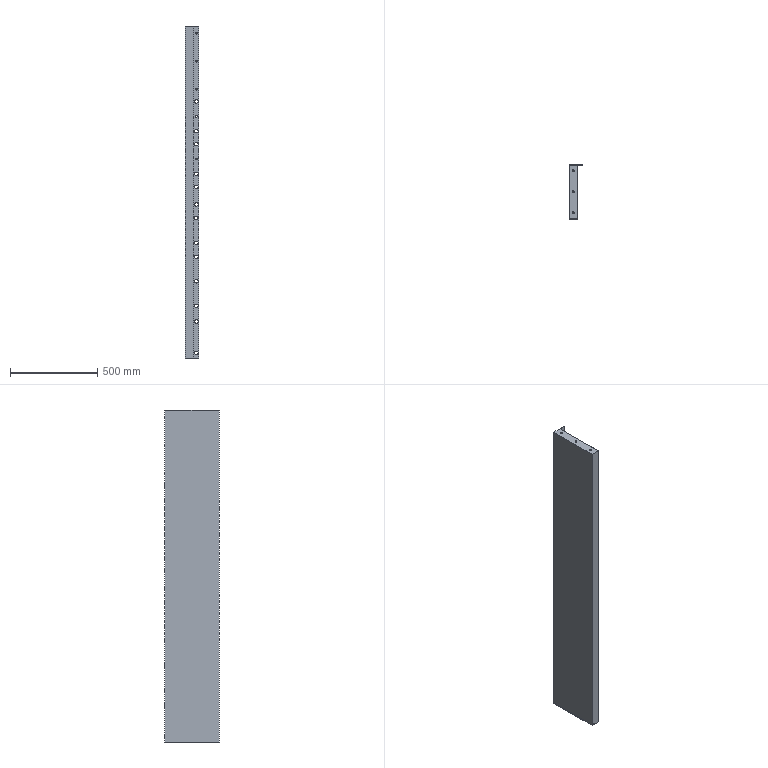Part | SolidWorks | features BaseBody 1 | 1 solid | 60 faces | box 80 x 310 x 1900 mm | volume 2544201 mm3 | cylinder 48 | plane 12 | commonest cylinder face diameters 20 x26 11 x16 10.6 x6